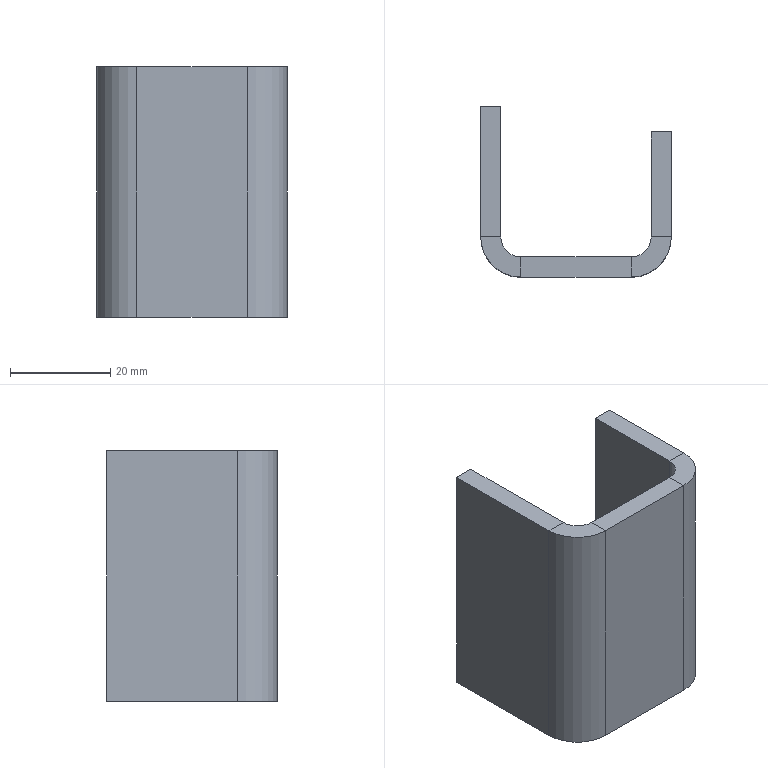Part | STEP file | 06-Reinforcing bent plate 1 | 1 solid | 22 faces | box 38 x 34 x 50 mm | volume 17557 mm3 | plane 18 | cylinder 4 | commonest cylinder face diameters 8 x2 16 x2
STEP:
#1=CARTESIAN_POINT('',(0.,0.,0.));
#2=DIRECTION('',(0.,0.,1.));
#3=DIRECTION('',(1.,0.,0.));
#4=AXIS2_PLACEMENT_3D('',#1,#2,#3);
#5=CARTESIAN_POINT('',(0.,-26.,50.));
#6=VERTEX_POINT('',#5);
#7=CARTESIAN_POINT('',(4.,-26.,50.));
#8=VERTEX_POINT('',#7);
#9=CARTESIAN_POINT('',(0.,-26.,50.));
#10=DIRECTION('',(1.,0.,0.));
#11=VECTOR('',#10,1.);
#12=LINE('',#9,#11);
#13=CARTESIAN_POINT('',(0.,-26.,50.));
#14=DIRECTION('',(0.,0.,1.));
#15=DIRECTION('',(1.,0.,0.));
#16=AXIS2_PLACEMENT_3D('',#13,#14,#15);
#17=PLANE('',#16);
#18=CARTESIAN_POINT('',(0.,0.));
#19=DIRECTION('',(1.,0.));
#20=VECTOR('',#19,1.);
#21=LINE('',#18,#20);
#22=(GEOMETRIC_REPRESENTATION_CONTEXT(2)PARAMETRIC_REPRESENTATION_CONTEXT()REPRESENTATION_CONTEXT('',''));
#23=DEFINITIONAL_REPRESENTATION('',(#21),#22);
#24=PCURVE('',#17,#23);
#25=CARTESIAN_POINT('',(8.,-30.,50.));
#26=DIRECTION('',(0.,0.,1.));
#27=DIRECTION('',(1.,0.,0.));
#28=AXIS2_PLACEMENT_3D('',#25,#26,#27);
#29=PLANE('',#28);
#30=CARTESIAN_POINT('',(-8.,4.));
#31=DIRECTION('',(1.,0.));
#32=VECTOR('',#31,1.);
#33=LINE('',#30,#32);
#34=(GEOMETRIC_REPRESENTATION_CONTEXT(2)PARAMETRIC_REPRESENTATION_CONTEXT()REPRESENTATION_CONTEXT('',''));
#35=DEFINITIONAL_REPRESENTATION('',(#33),#34);
#36=PCURVE('',#29,#35);
#37=SURFACE_CURVE('',#12,(#24,#36),.PCURVE_S1.);
#38=EDGE_CURVE('',#6,#8,#37,.T.);
#39=ORIENTED_EDGE('',*,*,#38,.F.);
#40=CARTESIAN_POINT('',(8.,-34.,50.));
#41=VERTEX_POINT('',#40);
#42=CARTESIAN_POINT('',(8.,-26.,50.));
#43=DIRECTION('',(0.,0.,1.));
#44=DIRECTION('',(-1.,0.,0.));
#45=AXIS2_PLACEMENT_3D('',#42,#43,#44);
#46=CIRCLE('',#45,8.);
#47=CARTESIAN_POINT('',(8.,0.));
#48=DIRECTION('',(-1.,0.));
#49=AXIS2_PLACEMENT_2D('',#47,#48);
#50=CIRCLE('',#49,8.);
#51=(GEOMETRIC_REPRESENTATION_CONTEXT(2)PARAMETRIC_REPRESENTATION_CONTEXT()REPRESENTATION_CONTEXT('',''));
#52=DEFINITIONAL_REPRESENTATION('',(#50),#51);
#53=PCURVE('',#17,#52);
#54=CARTESIAN_POINT('',(8.,-26.,50.));
#55=DIRECTION('',(0.,0.,-1.));
#56=DIRECTION('',(-1.,0.,0.));
#57=AXIS2_PLACEMENT_3D('',#54,#55,#56);
#58=CYLINDRICAL_SURFACE('',#57,8.);
#59=CARTESIAN_POINT('',(6.283,0.));
#60=DIRECTION('',(-1.,0.));
#61=VECTOR('',#60,1.);
#62=LINE('',#59,#61);
#63=(GEOMETRIC_REPRESENTATION_CONTEXT(2)PARAMETRIC_REPRESENTATION_CONTEXT()REPRESENTATION_CONTEXT('',''));
#64=DEFINITIONAL_REPRESENTATION('',(#62),#63);
#65=PCURVE('',#58,#64);
#66=SURFACE_CURVE('',#46,(#53,#65),.PCURVE_S1.);
#67=EDGE_CURVE('',#6,#41,#66,.T.);
#68=ORIENTED_EDGE('',*,*,#67,.T.);
#69=CARTESIAN_POINT('',(8.,-30.,50.));
#70=VERTEX_POINT('',#69);
#71=CARTESIAN_POINT('',(8.,-30.,50.));
#72=DIRECTION('',(0.,-1.,0.));
#73=VECTOR('',#72,1.);
#74=LINE('',#71,#73);
#75=CARTESIAN_POINT('',(8.,-4.));
#76=DIRECTION('',(0.,-1.));
#77=VECTOR('',#76,1.);
#78=LINE('',#75,#77);
#79=(GEOMETRIC_REPRESENTATION_CONTEXT(2)PARAMETRIC_REPRESENTATION_CONTEXT()REPRESENTATION_CONTEXT('',''));
#80=DEFINITIONAL_REPRESENTATION('',(#78),#79);
#81=PCURVE('',#17,#80);
#82=CARTESIAN_POINT('',(34.,-26.,50.));
#83=DIRECTION('',(0.,0.,1.));
#84=DIRECTION('',(1.,0.,0.));
#85=AXIS2_PLACEMENT_3D('',#82,#83,#84);
#86=PLANE('',#85);
#87=CARTESIAN_POINT('',(-26.,-4.));
#88=DIRECTION('',(0.,-1.));
#89=VECTOR('',#88,1.);
#90=LINE('',#87,#89);
#91=(GEOMETRIC_REPRESENTATION_CONTEXT(2)PARAMETRIC_REPRESENTATION_CONTEXT()REPRESENTATION_CONTEXT('',''));
#92=DEFINITIONAL_REPRESENTATION('',(#90),#91);
#93=PCURVE('',#86,#92);
#94=SURFACE_CURVE('',#74,(#81,#93),.PCURVE_S1.);
#95=EDGE_CURVE('',#70,#41,#94,.T.);
#96=ORIENTED_EDGE('',*,*,#95,.F.);
#97=CARTESIAN_POINT('',(8.,-26.,50.));
#98=DIRECTION('',(0.,0.,1.));
#99=DIRECTION('',(1.,0.,0.));
#100=AXIS2_PLACEMENT_3D('',#97,#98,#99);
#101=CIRCLE('',#100,4.);
#102=CARTESIAN_POINT('',(8.,0.));
#103=DIRECTION('',(1.,0.));
#104=AXIS2_PLACEMENT_2D('',#102,#103);
#105=CIRCLE('',#104,4.);
#106=(GEOMETRIC_REPRESENTATION_CONTEXT(2)PARAMETRIC_REPRESENTATION_CONTEXT()REPRESENTATION_CONTEXT('',''));
#107=DEFINITIONAL_REPRESENTATION('',(#105),#106);
#108=PCURVE('',#17,#107);
#109=CARTESIAN_POINT('',(8.,-26.,50.));
#110=DIRECTION('',(0.,0.,-1.));
#111=DIRECTION('',(-1.,0.,0.));
#112=AXIS2_PLACEMENT_3D('',#109,#110,#111);
#113=CYLINDRICAL_SURFACE('',#112,4.);
#114=CARTESIAN_POINT('',(9.425,0.));
#115=DIRECTION('',(-1.,0.));
#116=VECTOR('',#115,1.);
#117=LINE('',#114,#116);
#118=(GEOMETRIC_REPRESENTATION_CONTEXT(2)PARAMETRIC_REPRESENTATION_CONTEXT()REPRESENTATION_CONTEXT('',''));
#119=DEFINITIONAL_REPRESENTATION('',(#117),#118);
#120=PCURVE('',#113,#119);
#121=SURFACE_CURVE('',#101,(#108,#120),.PCURVE_S1.);
#122=EDGE_CURVE('',#8,#70,#121,.T.);
#123=ORIENTED_EDGE('',*,*,#122,.F.);
#124=EDGE_LOOP('',(#39,#68,#96,#123));
#125=FACE_BOUND('',#124,.T.);
#126=ADVANCED_FACE('',(#125),#17,.T.);
#127=CARTESIAN_POINT('',(0.,0.,50.));
#128=VERTEX_POINT('',#127);
#129=CARTESIAN_POINT('',(0.,0.,50.));
#130=DIRECTION('',(0.,-1.,0.));
#131=VECTOR('',#130,1.);
#132=LINE('',#129,#131);
#133=CARTESIAN_POINT('',(-8.,30.));
#134=DIRECTION('',(0.,-1.));
#135=VECTOR('',#134,1.);
#136=LINE('',#133,#135);
#137=(GEOMETRIC_REPRESENTATION_CONTEXT(2)PARAMETRIC_REPRESENTATION_CONTEXT()REPRESENTATION_CONTEXT('',''));
#138=DEFINITIONAL_REPRESENTATION('',(#136),#137);
#139=PCURVE('',#29,#138);
#140=CARTESIAN_POINT('',(0.,0.,50.));
#141=DIRECTION('',(1.,0.,0.));
#142=DIRECTION('',(0.,1.,0.));
#143=AXIS2_PLACEMENT_3D('',#140,#141,#142);
#144=PLANE('',#143);
#145=CARTESIAN_POINT('',(0.,0.));
#146=DIRECTION('',(-1.,0.));
#147=VECTOR('',#146,1.);
#148=LINE('',#145,#147);
#149=(GEOMETRIC_REPRESENTATION_CONTEXT(2)PARAMETRIC_REPRESENTATION_CONTEXT()REPRESENTATION_CONTEXT('',''));
#150=DEFINITIONAL_REPRESENTATION('',(#148),#149);
#151=PCURVE('',#144,#150);
#152=SURFACE_CURVE('',#132,(#139,#151),.PCURVE_S1.);
#153=EDGE_CURVE('',#128,#6,#152,.T.);
#154=ORIENTED_EDGE('',*,*,#153,.T.);
#155=ORIENTED_EDGE('',*,*,#38,.T.);
#156=CARTESIAN_POINT('',(4.,0.,50.));
#157=VERTEX_POINT('',#156);
#158=CARTESIAN_POINT('',(4.,0.,50.));
#159=DIRECTION('',(0.,-1.,0.));
#160=VECTOR('',#159,1.);
#161=LINE('',#158,#160);
#162=CARTESIAN_POINT('',(-4.,30.));
#163=DIRECTION('',(0.,-1.));
#164=VECTOR('',#163,1.);
#165=LINE('',#162,#164);
#166=(GEOMETRIC_REPRESENTATION_CONTEXT(2)PARAMETRIC_REPRESENTATION_CONTEXT()REPRESENTATION_CONTEXT('',''));
#167=DEFINITIONAL_REPRESENTATION('',(#165),#166);
#168=PCURVE('',#29,#167);
#169=CARTESIAN_POINT('',(4.,0.,50.));
#170=DIRECTION('',(1.,0.,0.));
#171=DIRECTION('',(0.,1.,0.));
#172=AXIS2_PLACEMENT_3D('',#169,#170,#171);
#173=PLANE('',#172);
#174=CARTESIAN_POINT('',(0.,0.));
#175=DIRECTION('',(-1.,0.));
#176=VECTOR('',#175,1.);
#177=LINE('',#174,#176);
#178=(GEOMETRIC_REPRESENTATION_CONTEXT(2)PARAMETRIC_REPRESENTATION_CONTEXT()REPRESENTATION_CONTEXT('',''));
#179=DEFINITIONAL_REPRESENTATION('',(#177),#178);
#180=PCURVE('',#173,#179);
#181=SURFACE_CURVE('',#161,(#168,#180),.PCURVE_S1.);
#182=EDGE_CURVE('',#157,#8,#181,.T.);
#183=ORIENTED_EDGE('',*,*,#182,.F.);
#184=CARTESIAN_POINT('',(0.,0.,50.));
#185=DIRECTION('',(1.,0.,0.));
#186=VECTOR('',#185,1.);
#187=LINE('',#184,#186);
#188=CARTESIAN_POINT('',(-8.,30.));
#189=DIRECTION('',(1.,0.));
#190=VECTOR('',#189,1.);
#191=LINE('',#188,#190);
#192=(GEOMETRIC_REPRESENTATION_CONTEXT(2)PARAMETRIC_REPRESENTATION_CONTEXT()REPRESENTATION_CONTEXT('',''));
#193=DEFINITIONAL_REPRESENTATION('',(#191),#192);
#194=PCURVE('',#29,#193);
#195=CARTESIAN_POINT('',(0.,0.,50.));
#196=DIRECTION('',(0.,1.,0.));
#197=DIRECTION('',(-1.,0.,0.));
#198=AXIS2_PLACEMENT_3D('',#195,#196,#197);
#199=PLANE('',#198);
#200=CARTESIAN_POINT('',(0.,0.));
#201=DIRECTION('',(-1.,0.));
#202=VECTOR('',#201,1.);
#203=LINE('',#200,#202);
#204=(GEOMETRIC_REPRESENTATION_CONTEXT(2)PARAMETRIC_REPRESENTATION_CONTEXT()REPRESENTATION_CONTEXT('',''));
#205=DEFINITIONAL_REPRESENTATION('',(#203),#204);
#206=PCURVE('',#199,#205);
#207=SURFACE_CURVE('',#187,(#194,#206),.PCURVE_S1.);
#208=EDGE_CURVE('',#128,#157,#207,.T.);
#209=ORIENTED_EDGE('',*,*,#208,.F.);
#210=EDGE_LOOP('',(#154,#155,#183,#209));
#211=FACE_BOUND('',#210,.T.);
#212=ADVANCED_FACE('',(#211),#29,.T.);
#213=CARTESIAN_POINT('',(8.,-34.,0.));
#214=VERTEX_POINT('',#213);
#215=CARTESIAN_POINT('',(8.,-30.,0.));
#216=VERTEX_POINT('',#215);
#217=CARTESIAN_POINT('',(8.,-34.,0.));
#218=DIRECTION('',(0.,1.,0.));
#219=VECTOR('',#218,1.);
#220=LINE('',#217,#219);
#221=CARTESIAN_POINT('',(8.,-34.,0.));
#222=DIRECTION('',(0.,0.,-1.));
#223=DIRECTION('',(-1.,0.,0.));
#224=AXIS2_PLACEMENT_3D('',#221,#222,#223);
#225=PLANE('',#224);
#226=CARTESIAN_POINT('',(0.,0.));
#227=DIRECTION('',(0.,1.));
#228=VECTOR('',#227,1.);
#229=LINE('',#226,#228);
#230=(GEOMETRIC_REPRESENTATION_CONTEXT(2)PARAMETRIC_REPRESENTATION_CONTEXT()REPRESENTATION_CONTEXT('',''));
#231=DEFINITIONAL_REPRESENTATION('',(#229),#230);
#232=PCURVE('',#225,#231);
#233=CARTESIAN_POINT('',(4.,-26.,0.));
#234=DIRECTION('',(0.,0.,-1.));
#235=DIRECTION('',(-1.,0.,0.));
#236=AXIS2_PLACEMENT_3D('',#233,#234,#235);
#237=PLANE('',#236);
#238=CARTESIAN_POINT('',(-4.,-8.));
#239=DIRECTION('',(0.,1.));
#240=VECTOR('',#239,1.);
#241=LINE('',#238,#240);
#242=(GEOMETRIC_REPRESENTATION_CONTEXT(2)PARAMETRIC_REPRESENTATION_CONTEXT()REPRESENTATION_CONTEXT('',''));
#243=DEFINITIONAL_REPRESENTATION('',(#241),#242);
#244=PCURVE('',#237,#243);
#245=SURFACE_CURVE('',#220,(#232,#244),.PCURVE_S1.);
#246=EDGE_CURVE('',#214,#216,#245,.T.);
#247=ORIENTED_EDGE('',*,*,#246,.F.);
#248=CARTESIAN_POINT('',(0.,-26.,0.));
#249=VERTEX_POINT('',#248);
#250=CARTESIAN_POINT('',(8.,-26.,0.));
#251=DIRECTION('',(0.,0.,1.));
#252=DIRECTION('',(-1.,0.,0.));
#253=AXIS2_PLACEMENT_3D('',#250,#251,#252);
#254=CIRCLE('',#253,8.);
#255=CARTESIAN_POINT('',(8.,8.));
#256=CARTESIAN_POINT('',(8.,-5.856));
#257=CARTESIAN_POINT('',(-4.,1.072));
#258=CARTESIAN_POINT('',(-16.,8.));
#259=CARTESIAN_POINT('',(-4.,14.928));
#260=CARTESIAN_POINT('',(8.,21.856));
#261=CARTESIAN_POINT('',(8.,8.));
#262=(BOUNDED_CURVE()B_SPLINE_CURVE(2,(#255,#256,#257,#258,#259,#260,#261),.UNSPECIFIED.,.T.,.F.)B_SPLINE_CURVE_WITH_KNOTS((1,2,2,2,2,1),(-2.094,0.,2.094,4.189,6.283,8.378),.UNSPECIFIED.)CURVE()GEOMETRIC_REPRESENTATION_ITEM()RATIONAL_B_SPLINE_CURVE((1.,0.5,1.,0.5,1.,0.5,1.))REPRESENTATION_ITEM(''));
#263=(GEOMETRIC_REPRESENTATION_CONTEXT(2)PARAMETRIC_REPRESENTATION_CONTEXT()REPRESENTATION_CONTEXT('',''));
#264=DEFINITIONAL_REPRESENTATION('',(#262),#263);
#265=PCURVE('',#225,#264);
#266=CARTESIAN_POINT('',(6.283,50.));
#267=DIRECTION('',(-1.,0.));
#268=VECTOR('',#267,1.);
#269=LINE('',#266,#268);
#270=(GEOMETRIC_REPRESENTATION_CONTEXT(2)PARAMETRIC_REPRESENTATION_CONTEXT()REPRESENTATION_CONTEXT('',''));
#271=DEFINITIONAL_REPRESENTATION('',(#269),#270);
#272=PCURVE('',#58,#271);
#273=SURFACE_CURVE('',#254,(#265,#272),.PCURVE_S1.);
#274=EDGE_CURVE('',#249,#214,#273,.T.);
#275=ORIENTED_EDGE('',*,*,#274,.F.);
#276=CARTESIAN_POINT('',(4.,-26.,0.));
#277=VERTEX_POINT('',#276);
#278=CARTESIAN_POINT('',(4.,-26.,0.));
#279=DIRECTION('',(-1.,0.,0.));
#280=VECTOR('',#279,1.);
#281=LINE('',#278,#280);
#282=CARTESIAN_POINT('',(4.,8.));
#283=DIRECTION('',(1.,0.));
#284=VECTOR('',#283,1.);
#285=LINE('',#282,#284);
#286=(GEOMETRIC_REPRESENTATION_CONTEXT(2)PARAMETRIC_REPRESENTATION_CONTEXT()REPRESENTATION_CONTEXT('',''));
#287=DEFINITIONAL_REPRESENTATION('',(#285),#286);
#288=PCURVE('',#225,#287);
#289=CARTESIAN_POINT('',(30.,-26.,0.));
#290=DIRECTION('',(0.,0.,1.));
#291=DIRECTION('',(1.,0.,0.));
#292=AXIS2_PLACEMENT_3D('',#289,#290,#291);
#293=PLANE('',#292);
#294=CARTESIAN_POINT('',(-26.,0.));
#295=DIRECTION('',(-1.,0.));
#296=VECTOR('',#295,1.);
#297=LINE('',#294,#296);
#298=(GEOMETRIC_REPRESENTATION_CONTEXT(2)PARAMETRIC_REPRESENTATION_CONTEXT()REPRESENTATION_CONTEXT('',''));
#299=DEFINITIONAL_REPRESENTATION('',(#297),#298);
#300=PCURVE('',#293,#299);
#301=SURFACE_CURVE('',#281,(#288,#300),.PCURVE_S1.);
#302=EDGE_CURVE('',#277,#249,#301,.T.);
#303=ORIENTED_EDGE('',*,*,#302,.F.);
#304=CARTESIAN_POINT('',(8.,-26.,0.));
#305=DIRECTION('',(0.,0.,1.));
#306=DIRECTION('',(1.,0.,0.));
#307=AXIS2_PLACEMENT_3D('',#304,#305,#306);
#308=CIRCLE('',#307,4.);
#309=CARTESIAN_POINT('',(-4.,8.));
#310=CARTESIAN_POINT('',(-4.,14.928));
#311=CARTESIAN_POINT('',(2.,11.464));
#312=CARTESIAN_POINT('',(8.,8.));
#313=CARTESIAN_POINT('',(2.,4.536));
#314=CARTESIAN_POINT('',(-4.,1.072));
#315=CARTESIAN_POINT('',(-4.,8.));
#316=(BOUNDED_CURVE()B_SPLINE_CURVE(2,(#309,#310,#311,#312,#313,#314,#315),.UNSPECIFIED.,.T.,.F.)B_SPLINE_CURVE_WITH_KNOTS((1,2,2,2,2,1),(-2.094,0.,2.094,4.189,6.283,8.378),.UNSPECIFIED.)CURVE()GEOMETRIC_REPRESENTATION_ITEM()RATIONAL_B_SPLINE_CURVE((1.,0.5,1.,0.5,1.,0.5,1.))REPRESENTATION_ITEM(''));
#317=(GEOMETRIC_REPRESENTATION_CONTEXT(2)PARAMETRIC_REPRESENTATION_CONTEXT()REPRESENTATION_CONTEXT('',''));
#318=DEFINITIONAL_REPRESENTATION('',(#316),#317);
#319=PCURVE('',#225,#318);
#320=CARTESIAN_POINT('',(9.425,50.));
#321=DIRECTION('',(-1.,0.));
#322=VECTOR('',#321,1.);
#323=LINE('',#320,#322);
#324=(GEOMETRIC_REPRESENTATION_CONTEXT(2)PARAMETRIC_REPRESENTATION_CONTEXT()REPRESENTATION_CONTEXT('',''));
#325=DEFINITIONAL_REPRESENTATION('',(#323),#324);
#326=PCURVE('',#113,#325);
#327=SURFACE_CURVE('',#308,(#319,#326),.PCURVE_S1.);
#328=EDGE_CURVE('',#277,#216,#327,.T.);
#329=ORIENTED_EDGE('',*,*,#328,.T.);
#330=EDGE_LOOP('',(#247,#275,#303,#329));
#331=FACE_BOUND('',#330,.T.);
#332=ADVANCED_FACE('',(#331),#225,.T.);
#333=CARTESIAN_POINT('',(30.,-34.,0.));
#334=VERTEX_POINT('',#333);
#335=CARTESIAN_POINT('',(0.,-34.,0.));
#336=DIRECTION('',(1.,0.,0.));
#337=VECTOR('',#336,1.);
#338=LINE('',#335,#337);
#339=CARTESIAN_POINT('',(4.,-8.));
#340=DIRECTION('',(-1.,0.));
#341=VECTOR('',#340,1.);
#342=LINE('',#339,#341);
#343=(GEOMETRIC_REPRESENTATION_CONTEXT(2)PARAMETRIC_REPRESENTATION_CONTEXT()REPRESENTATION_CONTEXT('',''));
#344=DEFINITIONAL_REPRESENTATION('',(#342),#343);
#345=PCURVE('',#237,#344);
#346=CARTESIAN_POINT('',(0.,-34.,50.));
#347=DIRECTION('',(0.,1.,0.));
#348=DIRECTION('',(0.,0.,1.));
#349=AXIS2_PLACEMENT_3D('',#346,#347,#348);
#350=PLANE('',#349);
#351=CARTESIAN_POINT('',(-50.,0.));
#352=DIRECTION('',(0.,1.));
#353=VECTOR('',#352,1.);
#354=LINE('',#351,#353);
#355=(GEOMETRIC_REPRESENTATION_CONTEXT(2)PARAMETRIC_REPRESENTATION_CONTEXT()REPRESENTATION_CONTEXT('',''));
#356=DEFINITIONAL_REPRESENTATION('',(#354),#355);
#357=PCURVE('',#350,#356);
#358=SURFACE_CURVE('',#338,(#345,#357),.PCURVE_S1.);
#359=EDGE_CURVE('',#214,#334,#358,.T.);
#360=ORIENTED_EDGE('',*,*,#359,.F.);
#361=ORIENTED_EDGE('',*,*,#246,.T.);
#362=CARTESIAN_POINT('',(30.,-30.,0.));
#363=VERTEX_POINT('',#362);
#364=CARTESIAN_POINT('',(0.,-30.,0.));
#365=DIRECTION('',(1.,0.,0.));
#366=VECTOR('',#365,1.);
#367=LINE('',#364,#366);
#368=CARTESIAN_POINT('',(4.,-4.));
#369=DIRECTION('',(-1.,0.));
#370=VECTOR('',#369,1.);
#371=LINE('',#368,#370);
#372=(GEOMETRIC_REPRESENTATION_CONTEXT(2)PARAMETRIC_REPRESENTATION_CONTEXT()REPRESENTATION_CONTEXT('',''));
#373=DEFINITIONAL_REPRESENTATION('',(#371),#372);
#374=PCURVE('',#237,#373);
#375=CARTESIAN_POINT('',(0.,-30.,50.));
#376=DIRECTION('',(0.,1.,0.));
#377=DIRECTION('',(0.,0.,1.));
#378=AXIS2_PLACEMENT_3D('',#375,#376,#377);
#379=PLANE('',#378);
#380=CARTESIAN_POINT('',(-50.,0.));
#381=DIRECTION('',(0.,1.));
#382=VECTOR('',#381,1.);
#383=LINE('',#380,#382);
#384=(GEOMETRIC_REPRESENTATION_CONTEXT(2)PARAMETRIC_REPRESENTATION_CONTEXT()REPRESENTATION_CONTEXT('',''));
#385=DEFINITIONAL_REPRESENTATION('',(#383),#384);
#386=PCURVE('',#379,#385);
#387=SURFACE_CURVE('',#367,(#374,#386),.PCURVE_S1.);
#388=EDGE_CURVE('',#216,#363,#387,.T.);
#389=ORIENTED_EDGE('',*,*,#388,.T.);
#390=CARTESIAN_POINT('',(30.,-30.,0.));
#391=DIRECTION('',(0.,-1.,0.));
#392=VECTOR('',#391,1.);
#393=LINE('',#390,#392);
#394=CARTESIAN_POINT('',(-26.,-4.));
#395=DIRECTION('',(0.,-1.));
#396=VECTOR('',#395,1.);
#397=LINE('',#394,#396);
#398=(GEOMETRIC_REPRESENTATION_CONTEXT(2)PARAMETRIC_REPRESENTATION_CONTEXT()REPRESENTATION_CONTEXT('',''));
#399=DEFINITIONAL_REPRESENTATION('',(#397),#398);
#400=PCURVE('',#237,#399);
#401=CARTESIAN_POINT('',(38.,-26.,0.));
#402=DIRECTION('',(0.,0.,-1.));
#403=DIRECTION('',(-1.,0.,0.));
#404=AXIS2_PLACEMENT_3D('',#401,#402,#403);
#405=PLANE('',#404);
#406=CARTESIAN_POINT('',(8.,-4.));
#407=DIRECTION('',(0.,-1.));
#408=VECTOR('',#407,1.);
#409=LINE('',#406,#408);
#410=(GEOMETRIC_REPRESENTATION_CONTEXT(2)PARAMETRIC_REPRESENTATION_CONTEXT()REPRESENTATION_CONTEXT('',''));
#411=DEFINITIONAL_REPRESENTATION('',(#409),#410);
#412=PCURVE('',#405,#411);
#413=SURFACE_CURVE('',#393,(#400,#412),.PCURVE_S1.);
#414=EDGE_CURVE('',#363,#334,#413,.T.);
#415=ORIENTED_EDGE('',*,*,#414,.T.);
#416=EDGE_LOOP('',(#360,#361,#389,#415));
#417=FACE_BOUND('',#416,.T.);
#418=ADVANCED_FACE('',(#417),#237,.T.);
#419=CARTESIAN_POINT('',(30.,-34.,50.));
#420=VERTEX_POINT('',#419);
#421=CARTESIAN_POINT('',(30.,-30.,50.));
#422=VERTEX_POINT('',#421);
#423=CARTESIAN_POINT('',(30.,-34.,50.));
#424=DIRECTION('',(0.,1.,0.));
#425=VECTOR('',#424,1.);
#426=LINE('',#423,#425);
#427=CARTESIAN_POINT('',(30.,-34.,50.));
#428=DIRECTION('',(0.,0.,1.));
#429=DIRECTION('',(1.,0.,0.));
#430=AXIS2_PLACEMENT_3D('',#427,#428,#429);
#431=PLANE('',#430);
#432=CARTESIAN_POINT('',(0.,0.));
#433=DIRECTION('',(0.,1.));
#434=VECTOR('',#433,1.);
#435=LINE('',#432,#434);
#436=(GEOMETRIC_REPRESENTATION_CONTEXT(2)PARAMETRIC_REPRESENTATION_CONTEXT()REPRESENTATION_CONTEXT('',''));
#437=DEFINITIONAL_REPRESENTATION('',(#435),#436);
#438=PCURVE('',#431,#437);
#439=CARTESIAN_POINT('',(-4.,-8.));
#440=DIRECTION('',(0.,1.));
#441=VECTOR('',#440,1.);
#442=LINE('',#439,#441);
#443=(GEOMETRIC_REPRESENTATION_CONTEXT(2)PARAMETRIC_REPRESENTATION_CONTEXT()REPRESENTATION_CONTEXT('',''));
#444=DEFINITIONAL_REPRESENTATION('',(#442),#443);
#445=PCURVE('',#86,#444);
#446=SURFACE_CURVE('',#426,(#438,#445),.PCURVE_S1.);
#447=EDGE_CURVE('',#420,#422,#446,.T.);
#448=ORIENTED_EDGE('',*,*,#447,.F.);
#449=CARTESIAN_POINT('',(38.,-26.,50.));
#450=VERTEX_POINT('',#449);
#451=CARTESIAN_POINT('',(30.,-26.,50.));
#452=DIRECTION('',(0.,0.,1.));
#453=DIRECTION('',(-1.,0.,0.));
#454=AXIS2_PLACEMENT_3D('',#451,#452,#453);
#455=CIRCLE('',#454,8.);
#456=CARTESIAN_POINT('',(0.,8.));
#457=DIRECTION('',(-1.,0.));
#458=AXIS2_PLACEMENT_2D('',#456,#457);
#459=CIRCLE('',#458,8.);
#460=(GEOMETRIC_REPRESENTATION_CONTEXT(2)PARAMETRIC_REPRESENTATION_CONTEXT()REPRESENTATION_CONTEXT('',''));
#461=DEFINITIONAL_REPRESENTATION('',(#459),#460);
#462=PCURVE('',#431,#461);
#463=CARTESIAN_POINT('',(30.,-26.,50.));
#464=DIRECTION('',(0.,0.,-1.));
#465=DIRECTION('',(-1.,0.,0.));
#466=AXIS2_PLACEMENT_3D('',#463,#464,#465);
#467=CYLINDRICAL_SURFACE('',#466,8.);
#468=CARTESIAN_POINT('',(6.283,0.));
#469=DIRECTION('',(-1.,0.));
#470=VECTOR('',#469,1.);
#471=LINE('',#468,#470);
#472=(GEOMETRIC_REPRESENTATION_CONTEXT(2)PARAMETRIC_REPRESENTATION_CONTEXT()REPRESENTATION_CONTEXT('',''));
#473=DEFINITIONAL_REPRESENTATION('',(#471),#472);
#474=PCURVE('',#467,#473);
#475=SURFACE_CURVE('',#455,(#462,#474),.PCURVE_S1.);
#476=EDGE_CURVE('',#420,#450,#475,.T.);
#477=ORIENTED_EDGE('',*,*,#476,.T.);
#478=CARTESIAN_POINT('',(34.,-26.,50.));
#479=VERTEX_POINT('',#478);
#480=CARTESIAN_POINT('',(34.,-26.,50.));
#481=DIRECTION('',(1.,0.,0.));
#482=VECTOR('',#481,1.);
#483=LINE('',#480,#482);
#484=CARTESIAN_POINT('',(4.,8.));
#485=DIRECTION('',(1.,0.));
#486=VECTOR('',#485,1.);
#487=LINE('',#484,#486);
#488=(GEOMETRIC_REPRESENTATION_CONTEXT(2)PARAMETRIC_REPRESENTATION_CONTEXT()REPRESENTATION_CONTEXT('',''));
#489=DEFINITIONAL_REPRESENTATION('',(#487),#488);
#490=PCURVE('',#431,#489);
#491=CARTESIAN_POINT('',(30.,-26.,50.));
#492=DIRECTION('',(0.,0.,1.));
#493=DIRECTION('',(1.,0.,0.));
#494=AXIS2_PLACEMENT_3D('',#491,#492,#493);
#495=PLANE('',#494);
#496=CARTESIAN_POINT('',(4.,0.));
#497=DIRECTION('',(1.,0.));
#498=VECTOR('',#497,1.);
#499=LINE('',#496,#498);
#500=(GEOMETRIC_REPRESENTATION_CONTEXT(2)PARAMETRIC_REPRESENTATION_CONTEXT()REPRESENTATION_CONTEXT('',''));
#501=DEFINITIONAL_REPRESENTATION('',(#499),#500);
#502=PCURVE('',#495,#501);
#503=SURFACE_CURVE('',#483,(#490,#502),.PCURVE_S1.);
#504=EDGE_CURVE('',#479,#450,#503,.T.);
#505=ORIENTED_EDGE('',*,*,#504,.F.);
#506=CARTESIAN_POINT('',(30.,-26.,50.));
#507=DIRECTION('',(0.,0.,1.));
#508=DIRECTION('',(1.,0.,0.));
#509=AXIS2_PLACEMENT_3D('',#506,#507,#508);
#510=CIRCLE('',#509,4.);
#511=CARTESIAN_POINT('',(0.,8.));
#512=DIRECTION('',(1.,0.));
#513=AXIS2_PLACEMENT_2D('',#511,#512);
#514=CIRCLE('',#513,4.);
#515=(GEOMETRIC_REPRESENTATION_CONTEXT(2)PARAMETRIC_REPRESENTATION_CONTEXT()REPRESENTATION_CONTEXT('',''));
#516=DEFINITIONAL_REPRESENTATION('',(#514),#515);
#517=PCURVE('',#431,#516);
#518=CARTESIAN_POINT('',(30.,-26.,50.));
#519=DIRECTION('',(0.,0.,-1.));
#520=DIRECTION('',(-1.,0.,0.));
#521=AXIS2_PLACEMENT_3D('',#518,#519,#520);
#522=CYLINDRICAL_SURFACE('',#521,4.);
#523=CARTESIAN_POINT('',(9.425,0.));
#524=DIRECTION('',(-1.,0.));
#525=VECTOR('',#524,1.);
#526=LINE('',#523,#525);
#527=(GEOMETRIC_REPRESENTATION_CONTEXT(2)PARAMETRIC_REPRESENTATION_CONTEXT()REPRESENTATION_CONTEXT('',''));
#528=DEFINITIONAL_REPRESENTATION('',(#526),#527);
#529=PCURVE('',#522,#528);
#530=SURFACE_CURVE('',#510,(#517,#529),.PCURVE_S1.);
#531=EDGE_CURVE('',#422,#479,#530,.T.);
#532=ORIENTED_EDGE('',*,*,#531,.F.);
#533=EDGE_LOOP('',(#448,#477,#505,#532));
#534=FACE_BOUND('',#533,.T.);
#535=ADVANCED_FACE('',(#534),#431,.T.);
#536=CARTESIAN_POINT('',(0.,-34.,50.));
#537=DIRECTION('',(1.,0.,0.));
#538=VECTOR('',#537,1.);
#539=LINE('',#536,#538);
#540=CARTESIAN_POINT('',(-34.,-8.));
#541=DIRECTION('',(1.,0.));
#542=VECTOR('',#541,1.);
#543=LINE('',#540,#542);
#544=(GEOMETRIC_REPRESENTATION_CONTEXT(2)PARAMETRIC_REPRESENTATION_CONTEXT()REPRESENTATION_CONTEXT('',''));
#545=DEFINITIONAL_REPRESENTATION('',(#543),#544);
#546=PCURVE('',#86,#545);
#547=CARTESIAN_POINT('',(0.,0.));
#548=DIRECTION('',(0.,1.));
#549=VECTOR('',#548,1.);
#550=LINE('',#547,#549);
#551=(GEOMETRIC_REPRESENTATION_CONTEXT(2)PARAMETRIC_REPRESENTATION_CONTEXT()REPRESENTATION_CONTEXT('',''));
#552=DEFINITIONAL_REPRESENTATION('',(#550),#551);
#553=PCURVE('',#350,#552);
#554=SURFACE_CURVE('',#539,(#546,#553),.PCURVE_S1.);
#555=EDGE_CURVE('',#41,#420,#554,.T.);
#556=ORIENTED_EDGE('',*,*,#555,.T.);
#557=ORIENTED_EDGE('',*,*,#447,.T.);
#558=CARTESIAN_POINT('',(0.,-30.,50.));
#559=DIRECTION('',(1.,0.,0.));
#560=VECTOR('',#559,1.);
#561=LINE('',#558,#560);
#562=CARTESIAN_POINT('',(-34.,-4.));
#563=DIRECTION('',(1.,0.));
#564=VECTOR('',#563,1.);
#565=LINE('',#562,#564);
#566=(GEOMETRIC_REPRESENTATION_CONTEXT(2)PARAMETRIC_REPRESENTATION_CONTEXT()REPRESENTATION_CONTEXT('',''));
#567=DEFINITIONAL_REPRESENTATION('',(#565),#566);
#568=PCURVE('',#86,#567);
#569=CARTESIAN_POINT('',(0.,0.));
#570=DIRECTION('',(0.,1.));
#571=VECTOR('',#570,1.);
#572=LINE('',#569,#571);
#573=(GEOMETRIC_REPRESENTATION_CONTEXT(2)PARAMETRIC_REPRESENTATION_CONTEXT()REPRESENTATION_CONTEXT('',''));
#574=DEFINITIONAL_REPRESENTATION('',(#572),#573);
#575=PCURVE('',#379,#574);
#576=SURFACE_CURVE('',#561,(#568,#575),.PCURVE_S1.);
#577=EDGE_CURVE('',#70,#422,#576,.T.);
#578=ORIENTED_EDGE('',*,*,#577,.F.);
#579=ORIENTED_EDGE('',*,*,#95,.T.);
#580=EDGE_LOOP('',(#556,#557,#578,#579));
#581=FACE_BOUND('',#580,.T.);
#582=ADVANCED_FACE('',(#581),#86,.T.);
#583=CARTESIAN_POINT('',(38.,-26.,0.));
#584=VERTEX_POINT('',#583);
#585=CARTESIAN_POINT('',(34.,-26.,0.));
#586=VERTEX_POINT('',#585);
#587=CARTESIAN_POINT('',(38.,-26.,0.));
#588=DIRECTION('',(-1.,0.,0.));
#589=VECTOR('',#588,1.);
#590=LINE('',#587,#589);
#591=CARTESIAN_POINT('',(0.,0.));
#592=DIRECTION('',(1.,0.));
#593=VECTOR('',#592,1.);
#594=LINE('',#591,#593);
#595=(GEOMETRIC_REPRESENTATION_CONTEXT(2)PARAMETRIC_REPRESENTATION_CONTEXT()REPRESENTATION_CONTEXT('',''));
#596=DEFINITIONAL_REPRESENTATION('',(#594),#595);
#597=PCURVE('',#405,#596);
#598=CARTESIAN_POINT('',(30.,-30.,0.));
#599=DIRECTION('',(0.,0.,-1.));
#600=DIRECTION('',(-1.,0.,0.));
#601=AXIS2_PLACEMENT_3D('',#598,#599,#600);
#602=PLANE('',#601);
#603=CARTESIAN_POINT('',(-8.,4.));
#604=DIRECTION('',(1.,0.));
#605=VECTOR('',#604,1.);
#606=LINE('',#603,#605);
#607=(GEOMETRIC_REPRESENTATION_CONTEXT(2)PARAMETRIC_REPRESENTATION_CONTEXT()REPRESENTATION_CONTEXT('',''));
#608=DEFINITIONAL_REPRESENTATION('',(#606),#607);
#609=PCURVE('',#602,#608);
#610=SURFACE_CURVE('',#590,(#597,#609),.PCURVE_S1.);
#611=EDGE_CURVE('',#584,#586,#610,.T.);
#612=ORIENTED_EDGE('',*,*,#611,.F.);
#613=CARTESIAN_POINT('',(30.,-26.,0.));
#614=DIRECTION('',(0.,0.,1.));
#615=DIRECTION('',(-1.,0.,0.));
#616=AXIS2_PLACEMENT_3D('',#613,#614,#615);
#617=CIRCLE('',#616,8.);
#618=CARTESIAN_POINT('',(16.,0.));
#619=CARTESIAN_POINT('',(16.,-13.856));
#620=CARTESIAN_POINT('',(4.,-6.928));
#621=CARTESIAN_POINT('',(-8.,0.));
#622=CARTESIAN_POINT('',(4.,6.928));
#623=CARTESIAN_POINT('',(16.,13.856));
#624=CARTESIAN_POINT('',(16.,0.));
#625=(BOUNDED_CURVE()B_SPLINE_CURVE(2,(#618,#619,#620,#621,#622,#623,#624),.UNSPECIFIED.,.T.,.F.)B_SPLINE_CURVE_WITH_KNOTS((1,2,2,2,2,1),(-2.094,0.,2.094,4.189,6.283,8.378),.UNSPECIFIED.)CURVE()GEOMETRIC_REPRESENTATION_ITEM()RATIONAL_B_SPLINE_CURVE((1.,0.5,1.,0.5,1.,0.5,1.))REPRESENTATION_ITEM(''));
#626=(GEOMETRIC_REPRESENTATION_CONTEXT(2)PARAMETRIC_REPRESENTATION_CONTEXT()REPRESENTATION_CONTEXT('',''));
#627=DEFINITIONAL_REPRESENTATION('',(#625),#626);
#628=PCURVE('',#405,#627);
#629=CARTESIAN_POINT('',(6.283,50.));
#630=DIRECTION('',(-1.,0.));
#631=VECTOR('',#630,1.);
#632=LINE('',#629,#631);
#633=(GEOMETRIC_REPRESENTATION_CONTEXT(2)PARAMETRIC_REPRESENTATION_CONTEXT()REPRESENTATION_CONTEXT('',''));
#634=DEFINITIONAL_REPRESENTATION('',(#632),#633);
#635=PCURVE('',#467,#634);
#636=SURFACE_CURVE('',#617,(#628,#635),.PCURVE_S1.);
#637=EDGE_CURVE('',#334,#584,#636,.T.);
#638=ORIENTED_EDGE('',*,*,#637,.F.);
#639=ORIENTED_EDGE('',*,*,#414,.F.);
#640=CARTESIAN_POINT('',(30.,-26.,0.));
#641=DIRECTION('',(0.,0.,1.));
#642=DIRECTION('',(1.,0.,0.));
#643=AXIS2_PLACEMENT_3D('',#640,#641,#642);
#644=CIRCLE('',#643,4.);
#645=CARTESIAN_POINT('',(4.,0.));
#646=CARTESIAN_POINT('',(4.,6.928));
#647=CARTESIAN_POINT('',(10.,3.464));
#648=CARTESIAN_POINT('',(16.,0.));
#649=CARTESIAN_POINT('',(10.,-3.464));
#650=CARTESIAN_POINT('',(4.,-6.928));
#651=CARTESIAN_POINT('',(4.,0.));
#652=(BOUNDED_CURVE()B_SPLINE_CURVE(2,(#645,#646,#647,#648,#649,#650,#651),.UNSPECIFIED.,.T.,.F.)B_SPLINE_CURVE_WITH_KNOTS((1,2,2,2,2,1),(-2.094,0.,2.094,4.189,6.283,8.378),.UNSPECIFIED.)CURVE()GEOMETRIC_REPRESENTATION_ITEM()RATIONAL_B_SPLINE_CURVE((1.,0.5,1.,0.5,1.,0.5,1.))REPRESENTATION_ITEM(''));
#653=(GEOMETRIC_REPRESENTATION_CONTEXT(2)PARAMETRIC_REPRESENTATION_CONTEXT()REPRESENTATION_CONTEXT('',''));
#654=DEFINITIONAL_REPRESENTATION('',(#652),#653);
#655=PCURVE('',#405,#654);
#656=CARTESIAN_POINT('',(9.425,50.));
#657=DIRECTION('',(-1.,0.));
#658=VECTOR('',#657,1.);
#659=LINE('',#656,#658);
#660=(GEOMETRIC_REPRESENTATION_CONTEXT(2)PARAMETRIC_REPRESENTATION_CONTEXT()REPRESENTATION_CONTEXT('',''));
#661=DEFINITIONAL_REPRESENTATION('',(#659),#660);
#662=PCURVE('',#522,#661);
#663=SURFACE_CURVE('',#644,(#655,#662),.PCURVE_S1.);
#664=EDGE_CURVE('',#363,#586,#663,.T.);
#665=ORIENTED_EDGE('',*,*,#664,.T.);
#666=EDGE_LOOP('',(#612,#638,#639,#665));
#667=FACE_BOUND('',#666,.T.);
#668=ADVANCED_FACE('',(#667),#405,.T.);
#669=CARTESIAN_POINT('',(38.,-5.066,0.));
#670=VERTEX_POINT('',#669);
#671=CARTESIAN_POINT('',(38.,-34.,0.));
#672=DIRECTION('',(0.,1.,0.));
#673=VECTOR('',#672,1.);
#674=LINE('',#671,#673);
#675=CARTESIAN_POINT('',(-8.,-4.));
#676=DIRECTION('',(0.,1.));
#677=VECTOR('',#676,1.);
#678=LINE('',#675,#677);
#679=(GEOMETRIC_REPRESENTATION_CONTEXT(2)PARAMETRIC_REPRESENTATION_CONTEXT()REPRESENTATION_CONTEXT('',''));
#680=DEFINITIONAL_REPRESENTATION('',(#678),#679);
#681=PCURVE('',#602,#680);
#682=CARTESIAN_POINT('',(38.,-34.,50.));
#683=DIRECTION('',(-1.,0.,0.));
#684=DIRECTION('',(0.,0.,1.));
#685=AXIS2_PLACEMENT_3D('',#682,#683,#684);
#686=PLANE('',#685);
#687=CARTESIAN_POINT('',(-50.,0.));
#688=DIRECTION('',(0.,1.));
#689=VECTOR('',#688,1.);
#690=LINE('',#687,#689);
#691=(GEOMETRIC_REPRESENTATION_CONTEXT(2)PARAMETRIC_REPRESENTATION_CONTEXT()REPRESENTATION_CONTEXT('',''));
#692=DEFINITIONAL_REPRESENTATION('',(#690),#691);
#693=PCURVE('',#686,#692);
#694=SURFACE_CURVE('',#674,(#681,#693),.PCURVE_S1.);
#695=EDGE_CURVE('',#584,#670,#694,.T.);
#696=ORIENTED_EDGE('',*,*,#695,.F.);
#697=ORIENTED_EDGE('',*,*,#611,.T.);
#698=CARTESIAN_POINT('',(34.,-5.066,0.));
#699=VERTEX_POINT('',#698);
#700=CARTESIAN_POINT('',(34.,-34.,0.));
#701=DIRECTION('',(0.,1.,0.));
#702=VECTOR('',#701,1.);
#703=LINE('',#700,#702);
#704=CARTESIAN_POINT('',(-4.,-4.));
#705=DIRECTION('',(0.,1.));
#706=VECTOR('',#705,1.);
#707=LINE('',#704,#706);
#708=(GEOMETRIC_REPRESENTATION_CONTEXT(2)PARAMETRIC_REPRESENTATION_CONTEXT()REPRESENTATION_CONTEXT('',''));
#709=DEFINITIONAL_REPRESENTATION('',(#707),#708);
#710=PCURVE('',#602,#709);
#711=CARTESIAN_POINT('',(34.,-34.,50.));
#712=DIRECTION('',(-1.,0.,0.));
#713=DIRECTION('',(0.,0.,1.));
#714=AXIS2_PLACEMENT_3D('',#711,#712,#713);
#715=PLANE('',#714);
#716=CARTESIAN_POINT('',(-50.,0.));
#717=DIRECTION('',(0.,1.));
#718=VECTOR('',#717,1.);
#719=LINE('',#716,#718);
#720=(GEOMETRIC_REPRESENTATION_CONTEXT(2)PARAMETRIC_REPRESENTATION_CONTEXT()REPRESENTATION_CONTEXT('',''));
#721=DEFINITIONAL_REPRESENTATION('',(#719),#720);
#722=PCURVE('',#715,#721);
#723=SURFACE_CURVE('',#703,(#710,#722),.PCURVE_S1.);
#724=EDGE_CURVE('',#586,#699,#723,.T.);
#725=ORIENTED_EDGE('',*,*,#724,.T.);
#726=CARTESIAN_POINT('',(34.,-5.066,0.));
#727=DIRECTION('',(1.,0.,0.));
#728=VECTOR('',#727,1.);
#729=LINE('',#726,#728);
#730=CARTESIAN_POINT('',(-4.,24.934));
#731=DIRECTION('',(-1.,0.));
#732=VECTOR('',#731,1.);
#733=LINE('',#730,#732);
#734=(GEOMETRIC_REPRESENTATION_CONTEXT(2)PARAMETRIC_REPRESENTATION_CONTEXT()REPRESENTATION_CONTEXT('',''));
#735=DEFINITIONAL_REPRESENTATION('',(#733),#734);
#736=PCURVE('',#602,#735);
#737=CARTESIAN_POINT('',(34.,-5.066,50.));
#738=DIRECTION('',(0.,1.,0.));
#739=DIRECTION('',(0.,0.,1.));
#740=AXIS2_PLACEMENT_3D('',#737,#738,#739);
#741=PLANE('',#740);
#742=CARTESIAN_POINT('',(-50.,0.));
#743=DIRECTION('',(0.,1.));
#744=VECTOR('',#743,1.);
#745=LINE('',#742,#744);
#746=(GEOMETRIC_REPRESENTATION_CONTEXT(2)PARAMETRIC_REPRESENTATION_CONTEXT()REPRESENTATION_CONTEXT('',''));
#747=DEFINITIONAL_REPRESENTATION('',(#745),#746);
#748=PCURVE('',#741,#747);
#749=SURFACE_CURVE('',#729,(#736,#748),.PCURVE_S1.);
#750=EDGE_CURVE('',#699,#670,#749,.T.);
#751=ORIENTED_EDGE('',*,*,#750,.T.);
#752=EDGE_LOOP('',(#696,#697,#725,#751));
#753=FACE_BOUND('',#752,.T.);
#754=ADVANCED_FACE('',(#753),#602,.T.);
#755=ORIENTED_EDGE('',*,*,#695,.T.);
#756=CARTESIAN_POINT('',(38.,-5.066,50.));
#757=VERTEX_POINT('',#756);
#758=CARTESIAN_POINT('',(38.,-5.066,50.));
#759=DIRECTION('',(0.,0.,-1.));
#760=VECTOR('',#759,1.);
#761=LINE('',#758,#760);
#762=CARTESIAN_POINT('',(0.,28.934));
#763=DIRECTION('',(-1.,0.));
#764=VECTOR('',#763,1.);
#765=LINE('',#762,#764);
#766=(GEOMETRIC_REPRESENTATION_CONTEXT(2)PARAMETRIC_REPRESENTATION_CONTEXT()REPRESENTATION_CONTEXT('',''));
#767=DEFINITIONAL_REPRESENTATION('',(#765),#766);
#768=PCURVE('',#686,#767);
#769=CARTESIAN_POINT('',(0.,4.));
#770=DIRECTION('',(-1.,0.));
#771=VECTOR('',#770,1.);
#772=LINE('',#769,#771);
#773=(GEOMETRIC_REPRESENTATION_CONTEXT(2)PARAMETRIC_REPRESENTATION_CONTEXT()REPRESENTATION_CONTEXT('',''));
#774=DEFINITIONAL_REPRESENTATION('',(#772),#773);
#775=PCURVE('',#741,#774);
#776=SURFACE_CURVE('',#761,(#768,#775),.PCURVE_S1.);
#777=EDGE_CURVE('',#757,#670,#776,.T.);
#778=ORIENTED_EDGE('',*,*,#777,.F.);
#779=CARTESIAN_POINT('',(38.,-34.,50.));
#780=DIRECTION('',(0.,1.,0.));
#781=VECTOR('',#780,1.);
#782=LINE('',#779,#781);
#783=CARTESIAN_POINT('',(0.,0.));
#784=DIRECTION('',(0.,1.));
#785=VECTOR('',#784,1.);
#786=LINE('',#783,#785);
#787=(GEOMETRIC_REPRESENTATION_CONTEXT(2)PARAMETRIC_REPRESENTATION_CONTEXT()REPRESENTATION_CONTEXT('',''));
#788=DEFINITIONAL_REPRESENTATION('',(#786),#787);
#789=PCURVE('',#686,#788);
#790=CARTESIAN_POINT('',(8.,-8.));
#791=DIRECTION('',(0.,1.));
#792=VECTOR('',#791,1.);
#793=LINE('',#790,#792);
#794=(GEOMETRIC_REPRESENTATION_CONTEXT(2)PARAMETRIC_REPRESENTATION_CONTEXT()REPRESENTATION_CONTEXT('',''));
#795=DEFINITIONAL_REPRESENTATION('',(#793),#794);
#796=PCURVE('',#495,#795);
#797=SURFACE_CURVE('',#782,(#789,#796),.PCURVE_S1.);
#798=EDGE_CURVE('',#450,#757,#797,.T.);
#799=ORIENTED_EDGE('',*,*,#798,.F.);
#800=CARTESIAN_POINT('',(38.,-26.,50.));
#801=DIRECTION('',(0.,0.,-1.));
#802=VECTOR('',#801,1.);
#803=LINE('',#800,#802);
#804=CARTESIAN_POINT('',(0.,8.));
#805=DIRECTION('',(-1.,0.));
#806=VECTOR('',#805,1.);
#807=LINE('',#804,#806);
#808=(GEOMETRIC_REPRESENTATION_CONTEXT(2)PARAMETRIC_REPRESENTATION_CONTEXT()REPRESENTATION_CONTEXT('',''));
#809=DEFINITIONAL_REPRESENTATION('',(#807),#808);
#810=PCURVE('',#686,#809);
#811=CARTESIAN_POINT('',(3.142,0.));
#812=DIRECTION('',(0.,1.));
#813=VECTOR('',#812,1.);
#814=LINE('',#811,#813);
#815=(GEOMETRIC_REPRESENTATION_CONTEXT(2)PARAMETRIC_REPRESENTATION_CONTEXT()REPRESENTATION_CONTEXT('',''));
#816=DEFINITIONAL_REPRESENTATION('',(#814),#815);
#817=PCURVE('',#467,#816);
#818=SURFACE_CURVE('',#803,(#810,#817),.PCURVE_S1.);
#819=EDGE_CURVE('',#450,#584,#818,.T.);
#820=ORIENTED_EDGE('',*,*,#819,.T.);
#821=EDGE_LOOP('',(#755,#778,#799,#820));
#822=FACE_BOUND('',#821,.T.);
#823=ADVANCED_FACE('',(#822),#686,.F.);
#824=ORIENTED_EDGE('',*,*,#750,.F.);
#825=CARTESIAN_POINT('',(34.,-5.066,50.));
#826=VERTEX_POINT('',#825);
#827=CARTESIAN_POINT('',(34.,-5.066,50.));
#828=DIRECTION('',(0.,0.,-1.));
#829=VECTOR('',#828,1.);
#830=LINE('',#827,#829);
#831=CARTESIAN_POINT('',(0.,0.));
#832=DIRECTION('',(-1.,0.));
#833=VECTOR('',#832,1.);
#834=LINE('',#831,#833);
#835=(GEOMETRIC_REPRESENTATION_CONTEXT(2)PARAMETRIC_REPRESENTATION_CONTEXT()REPRESENTATION_CONTEXT('',''));
#836=DEFINITIONAL_REPRESENTATION('',(#834),#835);
#837=PCURVE('',#741,#836);
#838=CARTESIAN_POINT('',(0.,28.934));
#839=DIRECTION('',(-1.,0.));
#840=VECTOR('',#839,1.);
#841=LINE('',#838,#840);
#842=(GEOMETRIC_REPRESENTATION_CONTEXT(2)PARAMETRIC_REPRESENTATION_CONTEXT()REPRESENTATION_CONTEXT('',''));
#843=DEFINITIONAL_REPRESENTATION('',(#841),#842);
#844=PCURVE('',#715,#843);
#845=SURFACE_CURVE('',#830,(#837,#844),.PCURVE_S1.);
#846=EDGE_CURVE('',#826,#699,#845,.T.);
#847=ORIENTED_EDGE('',*,*,#846,.F.);
#848=CARTESIAN_POINT('',(34.,-5.066,50.));
#849=DIRECTION('',(1.,0.,0.));
#850=VECTOR('',#849,1.);
#851=LINE('',#848,#850);
#852=CARTESIAN_POINT('',(0.,0.));
#853=DIRECTION('',(0.,1.));
#854=VECTOR('',#853,1.);
#855=LINE('',#852,#854);
#856=(GEOMETRIC_REPRESENTATION_CONTEXT(2)PARAMETRIC_REPRESENTATION_CONTEXT()REPRESENTATION_CONTEXT('',''));
#857=DEFINITIONAL_REPRESENTATION('',(#855),#856);
#858=PCURVE('',#741,#857);
#859=CARTESIAN_POINT('',(4.,20.934));
#860=DIRECTION('',(1.,0.));
#861=VECTOR('',#860,1.);
#862=LINE('',#859,#861);
#863=(GEOMETRIC_REPRESENTATION_CONTEXT(2)PARAMETRIC_REPRESENTATION_CONTEXT()REPRESENTATION_CONTEXT('',''));
#864=DEFINITIONAL_REPRESENTATION('',(#862),#863);
#865=PCURVE('',#495,#864);
#866=SURFACE_CURVE('',#851,(#858,#865),.PCURVE_S1.);
#867=EDGE_CURVE('',#826,#757,#866,.T.);
#868=ORIENTED_EDGE('',*,*,#867,.T.);
#869=ORIENTED_EDGE('',*,*,#777,.T.);
#870=EDGE_LOOP('',(#824,#847,#868,#869));
#871=FACE_BOUND('',#870,.T.);
#872=ADVANCED_FACE('',(#871),#741,.T.);
#873=ORIENTED_EDGE('',*,*,#724,.F.);
#874=CARTESIAN_POINT('',(34.,-26.,50.));
#875=DIRECTION('',(0.,0.,-1.));
#876=VECTOR('',#875,1.);
#877=LINE('',#874,#876);
#878=CARTESIAN_POINT('',(0.,8.));
#879=DIRECTION('',(-1.,0.));
#880=VECTOR('',#879,1.);
#881=LINE('',#878,#880);
#882=(GEOMETRIC_REPRESENTATION_CONTEXT(2)PARAMETRIC_REPRESENTATION_CONTEXT()REPRESENTATION_CONTEXT('',''));
#883=DEFINITIONAL_REPRESENTATION('',(#881),#882);
#884=PCURVE('',#715,#883);
#885=CARTESIAN_POINT('',(3.142,0.));
#886=DIRECTION('',(0.,1.));
#887=VECTOR('',#886,1.);
#888=LINE('',#885,#887);
#889=(GEOMETRIC_REPRESENTATION_CONTEXT(2)PARAMETRIC_REPRESENTATION_CONTEXT()REPRESENTATION_CONTEXT('',''));
#890=DEFINITIONAL_REPRESENTATION('',(#888),#889);
#891=PCURVE('',#522,#890);
#892=SURFACE_CURVE('',#877,(#884,#891),.PCURVE_S1.);
#893=EDGE_CURVE('',#479,#586,#892,.T.);
#894=ORIENTED_EDGE('',*,*,#893,.F.);
#895=CARTESIAN_POINT('',(34.,-34.,50.));
#896=DIRECTION('',(0.,1.,0.));
#897=VECTOR('',#896,1.);
#898=LINE('',#895,#897);
#899=CARTESIAN_POINT('',(0.,0.));
#900=DIRECTION('',(0.,1.));
#901=VECTOR('',#900,1.);
#902=LINE('',#899,#901);
#903=(GEOMETRIC_REPRESENTATION_CONTEXT(2)PARAMETRIC_REPRESENTATION_CONTEXT()REPRESENTATION_CONTEXT('',''));
#904=DEFINITIONAL_REPRESENTATION('',(#902),#903);
#905=PCURVE('',#715,#904);
#906=CARTESIAN_POINT('',(4.,-8.));
#907=DIRECTION('',(0.,1.));
#908=VECTOR('',#907,1.);
#909=LINE('',#906,#908);
#910=(GEOMETRIC_REPRESENTATION_CONTEXT(2)PARAMETRIC_REPRESENTATION_CONTEXT()REPRESENTATION_CONTEXT('',''));
#911=DEFINITIONAL_REPRESENTATION('',(#909),#910);
#912=PCURVE('',#495,#911);
#913=SURFACE_CURVE('',#898,(#905,#912),.PCURVE_S1.);
#914=EDGE_CURVE('',#479,#826,#913,.T.);
#915=ORIENTED_EDGE('',*,*,#914,.T.);
#916=ORIENTED_EDGE('',*,*,#846,.T.);
#917=EDGE_LOOP('',(#873,#894,#915,#916));
#918=FACE_BOUND('',#917,.T.);
#919=ADVANCED_FACE('',(#918),#715,.T.);
#920=ORIENTED_EDGE('',*,*,#893,.F.);
#921=ORIENTED_EDGE('',*,*,#531,.F.);
#922=CARTESIAN_POINT('',(30.,-30.,50.));
#923=DIRECTION('',(0.,0.,-1.));
#924=VECTOR('',#923,1.);
#925=LINE('',#922,#924);
#926=CARTESIAN_POINT('',(4.712,0.));
#927=DIRECTION('',(0.,1.));
#928=VECTOR('',#927,1.);
#929=LINE('',#926,#928);
#930=(GEOMETRIC_REPRESENTATION_CONTEXT(2)PARAMETRIC_REPRESENTATION_CONTEXT()REPRESENTATION_CONTEXT('',''));
#931=DEFINITIONAL_REPRESENTATION('',(#929),#930);
#932=PCURVE('',#522,#931);
#933=CARTESIAN_POINT('',(0.,30.));
#934=DIRECTION('',(-1.,0.));
#935=VECTOR('',#934,1.);
#936=LINE('',#933,#935);
#937=(GEOMETRIC_REPRESENTATION_CONTEXT(2)PARAMETRIC_REPRESENTATION_CONTEXT()REPRESENTATION_CONTEXT('',''));
#938=DEFINITIONAL_REPRESENTATION('',(#936),#937);
#939=PCURVE('',#379,#938);
#940=SURFACE_CURVE('',#925,(#932,#939),.PCURVE_S1.);
#941=EDGE_CURVE('',#422,#363,#940,.T.);
#942=ORIENTED_EDGE('',*,*,#941,.T.);
#943=ORIENTED_EDGE('',*,*,#664,.T.);
#944=EDGE_LOOP('',(#920,#921,#942,#943));
#945=FACE_BOUND('',#944,.F.);
#946=ADVANCED_FACE('',(#945),#522,.F.);
#947=ORIENTED_EDGE('',*,*,#388,.F.);
#948=CARTESIAN_POINT('',(8.,-30.,50.));
#949=DIRECTION('',(0.,0.,-1.));
#950=VECTOR('',#949,1.);
#951=LINE('',#948,#950);
#952=CARTESIAN_POINT('',(0.,8.));
#953=DIRECTION('',(-1.,0.));
#954=VECTOR('',#953,1.);
#955=LINE('',#952,#954);
#956=(GEOMETRIC_REPRESENTATION_CONTEXT(2)PARAMETRIC_REPRESENTATION_CONTEXT()REPRESENTATION_CONTEXT('',''));
#957=DEFINITIONAL_REPRESENTATION('',(#955),#956);
#958=PCURVE('',#379,#957);
#959=CARTESIAN_POINT('',(4.712,0.));
#960=DIRECTION('',(0.,1.));
#961=VECTOR('',#960,1.);
#962=LINE('',#959,#961);
#963=(GEOMETRIC_REPRESENTATION_CONTEXT(2)PARAMETRIC_REPRESENTATION_CONTEXT()REPRESENTATION_CONTEXT('',''));
#964=DEFINITIONAL_REPRESENTATION('',(#962),#963);
#965=PCURVE('',#113,#964);
#966=SURFACE_CURVE('',#951,(#958,#965),.PCURVE_S1.);
#967=EDGE_CURVE('',#70,#216,#966,.T.);
#968=ORIENTED_EDGE('',*,*,#967,.F.);
#969=ORIENTED_EDGE('',*,*,#577,.T.);
#970=ORIENTED_EDGE('',*,*,#941,.T.);
#971=EDGE_LOOP('',(#947,#968,#969,#970));
#972=FACE_BOUND('',#971,.T.);
#973=ADVANCED_FACE('',(#972),#379,.T.);
#974=ORIENTED_EDGE('',*,*,#967,.F.);
#975=ORIENTED_EDGE('',*,*,#122,.F.);
#976=CARTESIAN_POINT('',(4.,-26.,50.));
#977=DIRECTION('',(0.,0.,-1.));
#978=VECTOR('',#977,1.);
#979=LINE('',#976,#978);
#980=CARTESIAN_POINT('',(6.283,0.));
#981=DIRECTION('',(0.,1.));
#982=VECTOR('',#981,1.);
#983=LINE('',#980,#982);
#984=(GEOMETRIC_REPRESENTATION_CONTEXT(2)PARAMETRIC_REPRESENTATION_CONTEXT()REPRESENTATION_CONTEXT('',''));
#985=DEFINITIONAL_REPRESENTATION('',(#983),#984);
#986=PCURVE('',#113,#985);
#987=CARTESIAN_POINT('',(-26.,0.));
#988=DIRECTION('',(0.,-1.));
#989=VECTOR('',#988,1.);
#990=LINE('',#987,#989);
#991=(GEOMETRIC_REPRESENTATION_CONTEXT(2)PARAMETRIC_REPRESENTATION_CONTEXT()REPRESENTATION_CONTEXT('',''));
#992=DEFINITIONAL_REPRESENTATION('',(#990),#991);
#993=PCURVE('',#173,#992);
#994=SURFACE_CURVE('',#979,(#986,#993),.PCURVE_S1.);
#995=EDGE_CURVE('',#8,#277,#994,.T.);
#996=ORIENTED_EDGE('',*,*,#995,.T.);
#997=ORIENTED_EDGE('',*,*,#328,.T.);
#998=EDGE_LOOP('',(#974,#975,#996,#997));
#999=FACE_BOUND('',#998,.F.);
#1000=ADVANCED_FACE('',(#999),#113,.F.);
#1001=CARTESIAN_POINT('',(4.,0.,0.));
#1002=VERTEX_POINT('',#1001);
#1003=CARTESIAN_POINT('',(4.,0.,0.));
#1004=DIRECTION('',(0.,-1.,0.));
#1005=VECTOR('',#1004,1.);
#1006=LINE('',#1003,#1005);
#1007=CARTESIAN_POINT('',(0.,-50.));
#1008=DIRECTION('',(-1.,0.));
#1009=VECTOR('',#1008,1.);
#1010=LINE('',#1007,#1009);
#1011=(GEOMETRIC_REPRESENTATION_CONTEXT(2)PARAMETRIC_REPRESENTATION_CONTEXT()REPRESENTATION_CONTEXT('',''));
#1012=DEFINITIONAL_REPRESENTATION('',(#1010),#1011);
#1013=PCURVE('',#173,#1012);
#1014=CARTESIAN_POINT('',(-26.,26.));
#1015=DIRECTION('',(0.,-1.));
#1016=VECTOR('',#1015,1.);
#1017=LINE('',#1014,#1016);
#1018=(GEOMETRIC_REPRESENTATION_CONTEXT(2)PARAMETRIC_REPRESENTATION_CONTEXT()REPRESENTATION_CONTEXT('',''));
#1019=DEFINITIONAL_REPRESENTATION('',(#1017),#1018);
#1020=PCURVE('',#293,#1019);
#1021=SURFACE_CURVE('',#1006,(#1013,#1020),.PCURVE_S1.);
#1022=EDGE_CURVE('',#1002,#277,#1021,.T.);
#1023=ORIENTED_EDGE('',*,*,#1022,.F.);
#1024=CARTESIAN_POINT('',(4.,0.,50.));
#1025=DIRECTION('',(0.,0.,-1.));
#1026=VECTOR('',#1025,1.);
#1027=LINE('',#1024,#1026);
#1028=CARTESIAN_POINT('',(0.,0.));
#1029=DIRECTION('',(0.,-1.));
#1030=VECTOR('',#1029,1.);
#1031=LINE('',#1028,#1030);
#1032=(GEOMETRIC_REPRESENTATION_CONTEXT(2)PARAMETRIC_REPRESENTATION_CONTEXT()REPRESENTATION_CONTEXT('',''));
#1033=DEFINITIONAL_REPRESENTATION('',(#1031),#1032);
#1034=PCURVE('',#173,#1033);
#1035=CARTESIAN_POINT('',(-4.,0.));
#1036=DIRECTION('',(0.,-1.));
#1037=VECTOR('',#1036,1.);
#1038=LINE('',#1035,#1037);
#1039=(GEOMETRIC_REPRESENTATION_CONTEXT(2)PARAMETRIC_REPRESENTATION_CONTEXT()REPRESENTATION_CONTEXT('',''));
#1040=DEFINITIONAL_REPRESENTATION('',(#1038),#1039);
#1041=PCURVE('',#199,#1040);
#1042=SURFACE_CURVE('',#1027,(#1034,#1041),.PCURVE_S1.);
#1043=EDGE_CURVE('',#157,#1002,#1042,.T.);
#1044=ORIENTED_EDGE('',*,*,#1043,.F.);
#1045=ORIENTED_EDGE('',*,*,#182,.T.);
#1046=ORIENTED_EDGE('',*,*,#995,.T.);
#1047=EDGE_LOOP('',(#1023,#1044,#1045,#1046));
#1048=FACE_BOUND('',#1047,.T.);
#1049=ADVANCED_FACE('',(#1048),#173,.T.);
#1050=CARTESIAN_POINT('',(0.,0.,0.));
#1051=VERTEX_POINT('',#1050);
#1052=CARTESIAN_POINT('',(0.,0.,0.));
#1053=DIRECTION('',(1.,0.,0.));
#1054=VECTOR('',#1053,1.);
#1055=LINE('',#1052,#1054);
#1056=CARTESIAN_POINT('',(0.,-50.));
#1057=DIRECTION('',(-1.,0.));
#1058=VECTOR('',#1057,1.);
#1059=LINE('',#1056,#1058);
#1060=(GEOMETRIC_REPRESENTATION_CONTEXT(2)PARAMETRIC_REPRESENTATION_CONTEXT()REPRESENTATION_CONTEXT('',''));
#1061=DEFINITIONAL_REPRESENTATION('',(#1059),#1060);
#1062=PCURVE('',#199,#1061);
#1063=CARTESIAN_POINT('',(-30.,26.));
#1064=DIRECTION('',(1.,0.));
#1065=VECTOR('',#1064,1.);
#1066=LINE('',#1063,#1065);
#1067=(GEOMETRIC_REPRESENTATION_CONTEXT(2)PARAMETRIC_REPRESENTATION_CONTEXT()REPRESENTATION_CONTEXT('',''));
#1068=DEFINITIONAL_REPRESENTATION('',(#1066),#1067);
#1069=PCURVE('',#293,#1068);
#1070=SURFACE_CURVE('',#1055,(#1062,#1069),.PCURVE_S1.);
#1071=EDGE_CURVE('',#1051,#1002,#1070,.T.);
#1072=ORIENTED_EDGE('',*,*,#1071,.F.);
#1073=CARTESIAN_POINT('',(0.,0.,50.));
#1074=DIRECTION('',(0.,0.,-1.));
#1075=VECTOR('',#1074,1.);
#1076=LINE('',#1073,#1075);
#1077=CARTESIAN_POINT('',(0.,0.));
#1078=DIRECTION('',(0.,-1.));
#1079=VECTOR('',#1078,1.);
#1080=LINE('',#1077,#1079);
#1081=(GEOMETRIC_REPRESENTATION_CONTEXT(2)PARAMETRIC_REPRESENTATION_CONTEXT()REPRESENTATION_CONTEXT('',''));
#1082=DEFINITIONAL_REPRESENTATION('',(#1080),#1081);
#1083=PCURVE('',#199,#1082);
#1084=CARTESIAN_POINT('',(0.,0.));
#1085=DIRECTION('',(0.,-1.));
#1086=VECTOR('',#1085,1.);
#1087=LINE('',#1084,#1086);
#1088=(GEOMETRIC_REPRESENTATION_CONTEXT(2)PARAMETRIC_REPRESENTATION_CONTEXT()REPRESENTATION_CONTEXT('',''));
#1089=DEFINITIONAL_REPRESENTATION('',(#1087),#1088);
#1090=PCURVE('',#144,#1089);
#1091=SURFACE_CURVE('',#1076,(#1083,#1090),.PCURVE_S1.);
#1092=EDGE_CURVE('',#128,#1051,#1091,.T.);
#1093=ORIENTED_EDGE('',*,*,#1092,.F.);
#1094=ORIENTED_EDGE('',*,*,#208,.T.);
#1095=ORIENTED_EDGE('',*,*,#1043,.T.);
#1096=EDGE_LOOP('',(#1072,#1093,#1094,#1095));
#1097=FACE_BOUND('',#1096,.T.);
#1098=ADVANCED_FACE('',(#1097),#199,.T.);
#1099=CARTESIAN_POINT('',(0.,0.,0.));
#1100=DIRECTION('',(0.,-1.,0.));
#1101=VECTOR('',#1100,1.);
#1102=LINE('',#1099,#1101);
#1103=CARTESIAN_POINT('',(0.,-50.));
#1104=DIRECTION('',(-1.,0.));
#1105=VECTOR('',#1104,1.);
#1106=LINE('',#1103,#1105);
#1107=(GEOMETRIC_REPRESENTATION_CONTEXT(2)PARAMETRIC_REPRESENTATION_CONTEXT()REPRESENTATION_CONTEXT('',''));
#1108=DEFINITIONAL_REPRESENTATION('',(#1106),#1107);
#1109=PCURVE('',#144,#1108);
#1110=CARTESIAN_POINT('',(-30.,26.));
#1111=DIRECTION('',(0.,-1.));
#1112=VECTOR('',#1111,1.);
#1113=LINE('',#1110,#1112);
#1114=(GEOMETRIC_REPRESENTATION_CONTEXT(2)PARAMETRIC_REPRESENTATION_CONTEXT()REPRESENTATION_CONTEXT('',''));
#1115=DEFINITIONAL_REPRESENTATION('',(#1113),#1114);
#1116=PCURVE('',#293,#1115);
#1117=SURFACE_CURVE('',#1102,(#1109,#1116),.PCURVE_S1.);
#1118=EDGE_CURVE('',#1051,#249,#1117,.T.);
#1119=ORIENTED_EDGE('',*,*,#1118,.T.);
#1120=CARTESIAN_POINT('',(0.,-26.,50.));
#1121=DIRECTION('',(0.,0.,-1.));
#1122=VECTOR('',#1121,1.);
#1123=LINE('',#1120,#1122);
#1124=CARTESIAN_POINT('',(-26.,0.));
#1125=DIRECTION('',(0.,-1.));
#1126=VECTOR('',#1125,1.);
#1127=LINE('',#1124,#1126);
#1128=(GEOMETRIC_REPRESENTATION_CONTEXT(2)PARAMETRIC_REPRESENTATION_CONTEXT()REPRESENTATION_CONTEXT('',''));
#1129=DEFINITIONAL_REPRESENTATION('',(#1127),#1128);
#1130=PCURVE('',#144,#1129);
#1131=CARTESIAN_POINT('',(6.283,0.));
#1132=DIRECTION('',(0.,1.));
#1133=VECTOR('',#1132,1.);
#1134=LINE('',#1131,#1133);
#1135=(GEOMETRIC_REPRESENTATION_CONTEXT(2)PARAMETRIC_REPRESENTATION_CONTEXT()REPRESENTATION_CONTEXT('',''));
#1136=DEFINITIONAL_REPRESENTATION('',(#1134),#1135);
#1137=PCURVE('',#58,#1136);
#1138=SURFACE_CURVE('',#1123,(#1130,#1137),.PCURVE_S1.);
#1139=EDGE_CURVE('',#6,#249,#1138,.T.);
#1140=ORIENTED_EDGE('',*,*,#1139,.F.);
#1141=ORIENTED_EDGE('',*,*,#153,.F.);
#1142=ORIENTED_EDGE('',*,*,#1092,.T.);
#1143=EDGE_LOOP('',(#1119,#1140,#1141,#1142));
#1144=FACE_BOUND('',#1143,.T.);
#1145=ADVANCED_FACE('',(#1144),#144,.F.);
#1146=ORIENTED_EDGE('',*,*,#274,.T.);
#1147=CARTESIAN_POINT('',(8.,-34.,50.));
#1148=DIRECTION('',(0.,0.,-1.));
#1149=VECTOR('',#1148,1.);
#1150=LINE('',#1147,#1149);
#1151=CARTESIAN_POINT('',(4.712,0.));
#1152=DIRECTION('',(0.,1.));
#1153=VECTOR('',#1152,1.);
#1154=LINE('',#1151,#1153);
#1155=(GEOMETRIC_REPRESENTATION_CONTEXT(2)PARAMETRIC_REPRESENTATION_CONTEXT()REPRESENTATION_CONTEXT('',''));
#1156=DEFINITIONAL_REPRESENTATION('',(#1154),#1155);
#1157=PCURVE('',#58,#1156);
#1158=CARTESIAN_POINT('',(0.,8.));
#1159=DIRECTION('',(-1.,0.));
#1160=VECTOR('',#1159,1.);
#1161=LINE('',#1158,#1160);
#1162=(GEOMETRIC_REPRESENTATION_CONTEXT(2)PARAMETRIC_REPRESENTATION_CONTEXT()REPRESENTATION_CONTEXT('',''));
#1163=DEFINITIONAL_REPRESENTATION('',(#1161),#1162);
#1164=PCURVE('',#350,#1163);
#1165=SURFACE_CURVE('',#1150,(#1157,#1164),.PCURVE_S1.);
#1166=EDGE_CURVE('',#41,#214,#1165,.T.);
#1167=ORIENTED_EDGE('',*,*,#1166,.F.);
#1168=ORIENTED_EDGE('',*,*,#67,.F.);
#1169=ORIENTED_EDGE('',*,*,#1139,.T.);
#1170=EDGE_LOOP('',(#1146,#1167,#1168,#1169));
#1171=FACE_BOUND('',#1170,.T.);
#1172=ADVANCED_FACE('',(#1171),#58,.T.);
#1173=ORIENTED_EDGE('',*,*,#359,.T.);
#1174=CARTESIAN_POINT('',(30.,-34.,50.));
#1175=DIRECTION('',(0.,0.,-1.));
#1176=VECTOR('',#1175,1.);
#1177=LINE('',#1174,#1176);
#1178=CARTESIAN_POINT('',(0.,30.));
#1179=DIRECTION('',(-1.,0.));
#1180=VECTOR('',#1179,1.);
#1181=LINE('',#1178,#1180);
#1182=(GEOMETRIC_REPRESENTATION_CONTEXT(2)PARAMETRIC_REPRESENTATION_CONTEXT()REPRESENTATION_CONTEXT('',''));
#1183=DEFINITIONAL_REPRESENTATION('',(#1181),#1182);
#1184=PCURVE('',#350,#1183);
#1185=CARTESIAN_POINT('',(4.712,0.));
#1186=DIRECTION('',(0.,1.));
#1187=VECTOR('',#1186,1.);
#1188=LINE('',#1185,#1187);
#1189=(GEOMETRIC_REPRESENTATION_CONTEXT(2)PARAMETRIC_REPRESENTATION_CONTEXT()REPRESENTATION_CONTEXT('',''));
#1190=DEFINITIONAL_REPRESENTATION('',(#1188),#1189);
#1191=PCURVE('',#467,#1190);
#1192=SURFACE_CURVE('',#1177,(#1184,#1191),.PCURVE_S1.);
#1193=EDGE_CURVE('',#420,#334,#1192,.T.);
#1194=ORIENTED_EDGE('',*,*,#1193,.F.);
#1195=ORIENTED_EDGE('',*,*,#555,.F.);
#1196=ORIENTED_EDGE('',*,*,#1166,.T.);
#1197=EDGE_LOOP('',(#1173,#1194,#1195,#1196));
#1198=FACE_BOUND('',#1197,.T.);
#1199=ADVANCED_FACE('',(#1198),#350,.F.);
#1200=ORIENTED_EDGE('',*,*,#637,.T.);
#1201=ORIENTED_EDGE('',*,*,#819,.F.);
#1202=ORIENTED_EDGE('',*,*,#476,.F.);
#1203=ORIENTED_EDGE('',*,*,#1193,.T.);
#1204=EDGE_LOOP('',(#1200,#1201,#1202,#1203));
#1205=FACE_BOUND('',#1204,.T.);
#1206=ADVANCED_FACE('',(#1205),#467,.T.);
#1207=ORIENTED_EDGE('',*,*,#798,.T.);
#1208=ORIENTED_EDGE('',*,*,#867,.F.);
#1209=ORIENTED_EDGE('',*,*,#914,.F.);
#1210=ORIENTED_EDGE('',*,*,#504,.T.);
#1211=EDGE_LOOP('',(#1207,#1208,#1209,#1210));
#1212=FACE_BOUND('',#1211,.T.);
#1213=ADVANCED_FACE('',(#1212),#495,.T.);
#1214=ORIENTED_EDGE('',*,*,#1022,.T.);
#1215=ORIENTED_EDGE('',*,*,#302,.T.);
#1216=ORIENTED_EDGE('',*,*,#1118,.F.);
#1217=ORIENTED_EDGE('',*,*,#1071,.T.);
#1218=EDGE_LOOP('',(#1214,#1215,#1216,#1217));
#1219=FACE_BOUND('',#1218,.T.);
#1220=ADVANCED_FACE('',(#1219),#293,.F.);
#1221=CLOSED_SHELL('',(#126,#212,#332,#418,#535,#582,#668,#754,#823,#872,#919,#946,#973,#1000,#1049,#1098,#1145,#1172,#1199,#1206,#1213,#1220));
#1222=MANIFOLD_SOLID_BREP('',#1221);
#1223=(LENGTH_UNIT()NAMED_UNIT(*)SI_UNIT(.MILLI.,.METRE.));
#1224=UNCERTAINTY_MEASURE_WITH_UNIT(LENGTH_MEASURE(0.0000001),#1223,'','');
#1225=(NAMED_UNIT(*)PLANE_ANGLE_UNIT()SI_UNIT($,.RADIAN.));
#1226=(NAMED_UNIT(*)SI_UNIT($,.STERADIAN.)SOLID_ANGLE_UNIT());
#1227=(GEOMETRIC_REPRESENTATION_CONTEXT(3)GLOBAL_UNCERTAINTY_ASSIGNED_CONTEXT((#1224))GLOBAL_UNIT_ASSIGNED_CONTEXT((#1223,#1225,#1226))REPRESENTATION_CONTEXT('',''));
#1228=ADVANCED_BREP_SHAPE_REPRESENTATION('',(#4,#1222),#1227);